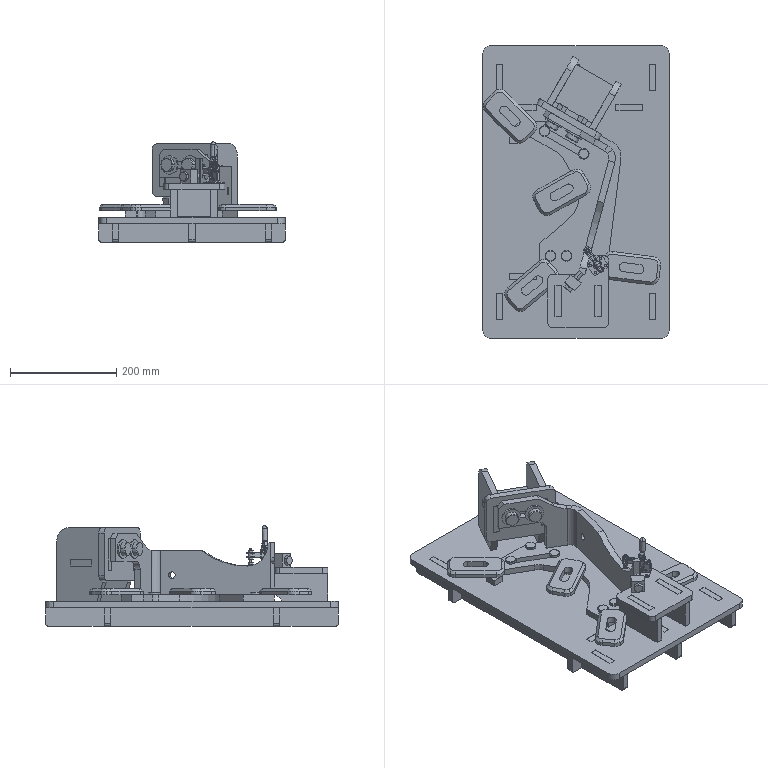Part | SolidWorks | features InContextFeatHolder 18, ReferencePattern 9, LocalLPattern 7, CosmeticWeldCutList 1 | 39 solids | 1097 faces | box 350 x 550 x 188.62 mm | volume 5135552 mm3 | plane 595 | cylinder 279 | cone 202 | sphere 18 | torus 2 | spline 1 | commonest cylinder face diameters 10.106 x32 3 x26 30 x25 20 x21 12.5 x20 10 x18